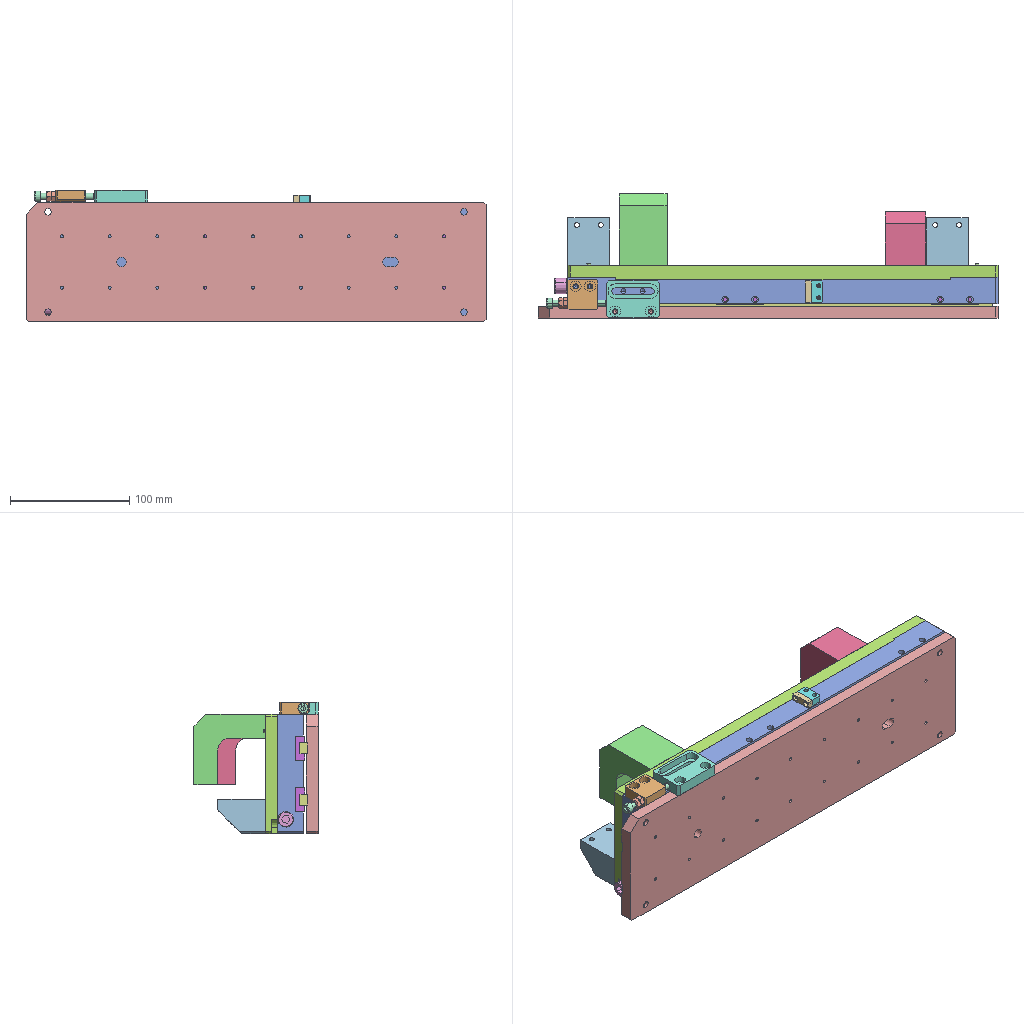Assembly | SolidWorks | 19 different items | 64 placed | box 385 x 104 x 110 mm
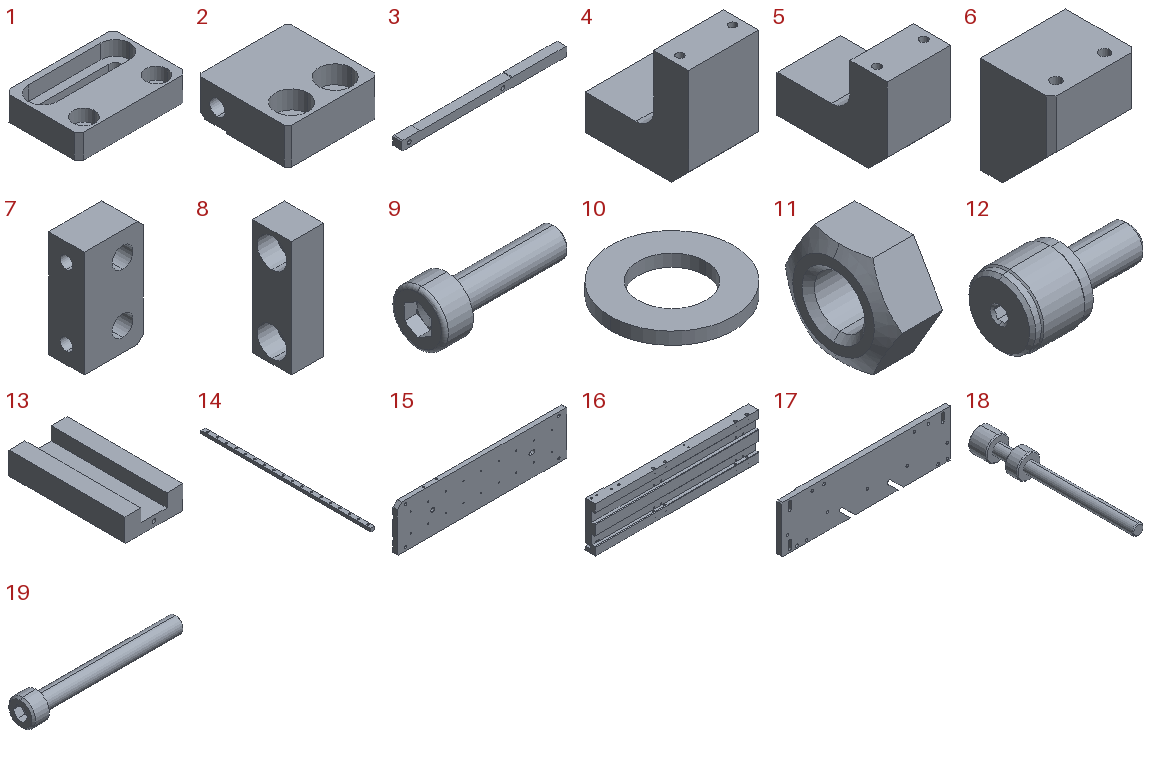Parts list (item | quantity | size | volume | features):
1 | x1 | 45 x 31 x 10 mm | 9481 mm3 | features ICE 4, Chamfer 1, Extrusion 1
2 | x1 | 25 x 25 x 10 mm | 4941 mm3 | features ICE 4, Chamfer 2, 3DProfileFeature 1, Extrusion 1, HoleWzd 1
3 | x1 | 180 x 9.8 x 10 mm | 15341 mm3 | features ICE 4, 3DProfileFeature 2, Chamfer 2, HoleWzd 2, Cut 1, Extrusion 1
4 | x1 | 40 x 59 x 60 mm | 77348 mm3 | features 3DProfileFeature 2, HoleWzd 2, Chamfer 1, Extrusion 1, Fillet 1, ICE 1
5 | x1 | 34 x 59 x 45 mm | 55439 mm3 | features 3DProfileFeature 2, HoleWzd 2, Chamfer 1, Extrusion 1, Fillet 1, ICE 1
6 | x2 | 35 x 29 x 40 mm | 32746 mm3 | features 3DProfileFeature 2, Chamfer 2, HoleWzd 2, Extrusion 1
7 | x1 | 10 x 6 x 18 mm | 923.956 mm3 | features 3DProfileFeature 1, Chamfer 1, Extrusion 1, HoleWzd 1, ICE 1
8 | x1 | 5 x 6 x 18 mm | 419.049 mm3 | features Cut 1, Extrusion 1, ICE 1
9 | x24 | 7.6 x 3 x 3 mm | 21.652 mm3 | features Fillet 2, RevCut 2, Boss 1, Chamfer 1, Cut 1, Extrusion 1, LPattern 1
10 | x16 | 10 x 10 x 1 mm | 54.782 mm3 | features Extrusion 1
11 | x2 | 4 x 9.238 x 8 mm | 160.7 mm3 | features ICE 1, RevCut 1, Revolution 1
12 | x2 | 15 x 8 x 8 mm | 435.538 mm3 | features BaseBody 1
13 | x4 | 20 x 39.9 x 8 mm | 4656 mm3 | features ICE 3, 3DProfileFeature 1, Chamfer 1, Extrusion 1, HoleWzd 1
14 | x2 | 9 x 360 x 6.5 mm | 18391 mm3 | features ICE 2, LPattern 2, Chamfer 1, Extrusion 1
15 | x1 | 385 x 10 x 100 mm | 371645 mm3 | features ICE 5, Chamfer 2, HoleWzd 2, 3DProfileFeature 1, Extrusion 1, LPattern 1
16 | x1 | 360 x 22 x 100 mm | 594910 mm3 | features ICE 9, HoleWzd 7, 3DProfileFeature 5, Chamfer 2, Fillet 2, Extrusion 1, LPattern 1, MirrorPattern 1
17 | x1 | 360 x 11.8 x 100 mm | 390446 mm3 | features ICE 12, Cut 3, Chamfer 1, Extrusion 1, LPattern 1
18 | x1 | 13 x 87 x 13 mm | 4026 mm3 | features ICE 5, Chamfer 1, Extrusion 1
19 | x1 | 50 x 8.5 x 8.5 mm | 1125 mm3 | features ICE 1, RevCut 1, Revolution 1
Mates (type | each side: item.copy, entity, surface, feature):
Coincident | 16.1 face plane Boss-Extrude1 | 17.1 face plane Boss-Extrude1 | 3 times
Coincident | 14.1 face plane Boss-Extrude1 | 13.1 face plane Cut-Extrude1 | 2 times
Coincident | 14.1 face plane Boss-Extrude1 | 13.2 face plane Cut-Extrude1
Coincident | 14.2 face plane Boss-Extrude1 | 13.3 face plane Cut-Extrude1 | 2 times
Coincident | 14.2 face plane Boss-Extrude1 | 13.4 face plane Cut-Extrude1 | 2 times
Coincident | 13.2 face plane Boss-Extrude1 | 13.4 face plane Boss-Extrude1 | 2 times
Coincident | 16.1 face plane Boss-Extrude1 | 2.1 face plane Boss-Extrude1 | 2 times
Coincident | 16.1 face plane Cut-Extrude2 | 2.1 face plane Boss-Extrude1
Concentric | 19.1 face cylinder Revolve1 | 11.1 face cylinder Cut-Revolve1
Concentric | 19.1 face cylinder Revolve1 | 11.2 face cylinder Cut-Revolve1
Concentric | 2.1 face cylinder M5 Tapped Hole1 | 19.1 face cylinder Revolve1
DistanceDim | 19.1 face plane Revolve1 | 2.1 face plane Boss-Extrude1
Coincident | 11.1 face plane Revolve1 | 11.2 face plane Revolve1
Coincident | 2.1 face plane Boss-Extrude1 | 11.1 face plane Revolve1
Coincident | 16.1 face plane Cut-Extrude5 | 18.1 face plane Boss-Extrude3
Coincident | 16.1 face plane Cut-Extrude4 | 3.1 face plane Boss-Extrude1 | 2 times
Concentric | 3.1 face cylinder M6 Tapped Hole1 | 18.1 face cylinder Boss-Extrude1
Coincident | 13.1 face plane Boss-Extrude1 | 13.3 face plane Boss-Extrude1
DistanceDim | 13.3 face plane Boss-Extrude1 | 16.1 face plane Boss-Extrude1
DistanceDim | 13.4 face plane Boss-Extrude1 | 13.3 face plane Boss-Extrude1
Concentric | 14.1 face cylinder LPattern2 | 9.1 face cylinder BaseBody
Coincident | 14.1 face plane LPattern2 | 9.1 face plane BaseHead
Concentric | 14.2 face cylinder LPattern1 | 9.2 face cylinder BaseBody
Coincident | 14.2 face plane LPattern2 | 9.2 face plane BaseHead
Coincident | 16.1 face plane Cut-Extrude8 | 10.1 face plane Base-Extrude
Concentric | 16.1 face cylinder Cut-Extrude8 | 10.1 face cylinder Base-Extrude
Coincident | 16.1 face plane Cut-Extrude8 | 10.2 face plane Base-Extrude
Concentric | 16.1 face cylinder Cut-Extrude8 | 10.2 face cylinder Base-Extrude
Coincident | 16.1 face plane Cut-Extrude8 | 10.3 face plane Base-Extrude
Concentric | 16.1 face cylinder Cut-Extrude8 | 10.3 face cylinder Base-Extrude
Coincident | 16.1 face plane Cut-Extrude8 | 10.4 face plane Base-Extrude
Concentric | 16.1 face cylinder LPattern1 | 10.4 face cylinder Base-Extrude
Coincident | 16.1 face plane Cut-Extrude8 | 10.5 face plane Base-Extrude
Concentric | 16.1 face cylinder LPattern1 | 10.5 face cylinder Base-Extrude
Coincident | 16.1 face plane Cut-Extrude8 | 10.6 face plane Base-Extrude
Concentric | 16.1 face cylinder Cut-Extrude8 | 10.6 face cylinder Base-Extrude
Coincident | 16.1 face plane Cut-Extrude8 | 10.7 face plane Base-Extrude
Concentric | 16.1 face cylinder Cut-Extrude8 | 10.7 face cylinder Base-Extrude
Coincident | 16.1 face plane Cut-Extrude8 | 10.8 face plane Base-Extrude | 2 times
Concentric | 16.1 face cylinder Cut-Extrude8 | 10.8 face cylinder Base-Extrude
Coincident | 16.1 face plane Cut-Extrude8 | 10.9 face plane Base-Extrude
Concentric | 16.1 face cylinder Cut-Extrude8 | 10.9 face cylinder Base-Extrude
Coincident | 16.1 face plane Cut-Extrude8 | 10.10 face plane Base-Extrude
Concentric | 16.1 face cylinder Cut-Extrude8 | 10.10 face cylinder Base-Extrude
Concentric | 16.1 face cylinder Cut-Extrude8 | 10.11 face cylinder Base-Extrude
Coincident | 16.1 face plane Cut-Extrude8 | 10.11 face plane Base-Extrude
Coincident | 16.1 face plane Cut-Extrude8 | 10.12 face plane Base-Extrude
Concentric | 16.1 face cylinder Cut-Extrude8 | 10.12 face cylinder Base-Extrude
Concentric | 16.1 face cylinder Cut-Extrude8 | 10.13 face cylinder Base-Extrude
Coincident | 16.1 face plane Cut-Extrude8 | 10.13 face plane Base-Extrude
Concentric | 16.1 face cylinder Cut-Extrude8 | 10.14 face cylinder Base-Extrude
Coincident | 16.1 face plane Cut-Extrude8 | 10.14 face plane Base-Extrude
Concentric | 16.1 face cylinder Cut-Extrude8 | 10.15 face cylinder Base-Extrude
Coincident | 16.1 face plane Cut-Extrude8 | 10.15 face plane Base-Extrude
Concentric | 16.1 face cylinder Cut-Extrude8 | 10.16 face cylinder Base-Extrude
Coincident | 16.1 face plane Cut-Extrude8 | 10.16 face plane Base-Extrude
Concentric | 10.15 face cylinder Base-Extrude | 9.3 face cylinder BaseBody
Coincident | 10.15 face plane Base-Extrude | 9.3 face plane BaseHead
Concentric | 16.1 face cylinder Cut-Extrude8 | 9.4 face cylinder BaseBody
Coincident | 10.16 face plane Base-Extrude | 9.4 face plane BaseHead
Concentric | 16.1 face cylinder Cut-Extrude8 | 9.5 face cylinder BaseBody
Coincident | 10.13 face plane Base-Extrude | 9.5 face plane BaseHead
Concentric | 16.1 face cylinder Cut-Extrude8 | 9.6 face cylinder BaseBody
Coincident | 10.14 face plane Base-Extrude | 9.6 face plane BaseHead
Concentric | 16.1 face cylinder Cut-Extrude8 | 9.7 face cylinder BaseBody
Coincident | 10.1 face plane Base-Extrude | 9.7 face plane BaseHead
Concentric | 16.1 face cylinder Cut-Extrude8 | 9.8 face cylinder BaseBody
Coincident | 10.11 face plane Base-Extrude | 9.8 face plane BaseHead
Concentric | 16.1 face cylinder Cut-Extrude8 | 9.9 face cylinder BaseBody
Coincident | 10.12 face plane Base-Extrude | 9.9 face plane BaseHead
Concentric | 16.1 face cylinder Cut-Extrude8 | 9.10 face cylinder BaseBody
Coincident | 10.2 face plane Base-Extrude | 9.10 face plane BaseHead
Concentric | 16.1 face cylinder LPattern1 | 9.11 face cylinder BaseBody
Coincident | 10.4 face plane Base-Extrude | 9.11 face plane BaseHead
Concentric | 10.3 face cylinder Base-Extrude | 9.12 face cylinder BaseBody
Coincident | 10.3 face plane Base-Extrude | 9.12 face plane BaseHead
Concentric | 16.1 face cylinder LPattern1 | 9.13 face cylinder BaseBody
Coincident | 10.5 face plane Base-Extrude | 9.13 face plane BaseHead
Concentric | 16.1 face cylinder Cut-Extrude8 | 9.14 face cylinder BaseBody
Coincident | 10.6 face plane Base-Extrude | 9.14 face plane BaseHead
Concentric | 16.1 face cylinder Cut-Extrude8 | 9.15 face cylinder BaseBody
Coincident | 10.8 face plane Base-Extrude | 9.15 face plane BaseHead
Concentric | 16.1 face cylinder Cut-Extrude8 | 9.16 face cylinder BaseBody
Coincident | 10.7 face plane Base-Extrude | 9.16 face plane BaseHead
Concentric | 10.10 face cylinder Base-Extrude | 9.17 face cylinder BaseBody
Coincident | 10.10 face plane Base-Extrude | 9.17 face plane BaseHead
Concentric | 16.1 face cylinder Cut-Extrude8 | 9.18 face cylinder BaseBody
Coincident | 10.9 face plane Base-Extrude | 9.18 face plane BaseHead
Coincident | 17.1 face plane Boss-Extrude1 | 4.1 face plane Boss-Extrude1 | 2 times
Concentric | 17.1 face cylinder Cut-Extrude4 | 5.1 face cylinder M5 Tapped Hole2 | 2 times
Coincident | 17.1 face plane Boss-Extrude1 | 5.1 face plane Boss-Extrude1
Concentric | 16.1 face cylinder M5 Tapped Hole1 | 9.19 face cylinder BaseBody
Concentric | 16.1 face cylinder M5 Tapped Hole2 | 9.20 face cylinder BaseBody
Concentric | 16.1 face cylinder M5 Tapped Hole3 | 9.21 face cylinder BaseBody
Coincident | 17.1 face plane Boss-Extrude1 | 9.21 face plane BaseHead
Coincident | 17.1 face plane Boss-Extrude1 | 9.20 face plane BaseHead
Coincident | 17.1 face plane Boss-Extrude1 | 9.19 face plane BaseHead
Concentric | 16.1 face cylinder M3 Tapped Hole1 | 9.22 face cylinder BaseBody
Coincident | 16.1 face plane Boss-Extrude1 | 9.22 face plane BaseHead
Concentric | 16.1 face cylinder M3 Tapped Hole1 | 9.23 face cylinder BaseBody
Coincident | 16.1 face plane Boss-Extrude1 | 9.23 face plane BaseHead
Coincident | 17.1 face plane Boss-Extrude1 | 6.1 face plane Boss-Extrude1 | 2 times
Coincident | 6.2 face plane Boss-Extrude1 | 6.1 face plane Boss-Extrude1
Concentric | 17.1 face cylinder Cut-Extrude6 | 6.2 face cylinder M5 Tapped Hole1 | 2 times
Coincident | 17.1 face plane Boss-Extrude1 | 6.2 face plane Boss-Extrude1
Coincident | 3.1 face plane Cut-Extrude4 | 12.1 face plane Input1
Concentric | 3.1 face cylinder Cut-Extrude5 | 12.1 face cylinder Input1
Coincident | 3.1 face plane Cut-Extrude4 | 12.2 face plane Input1
Concentric | 3.1 face cylinder Cut-Extrude5 | 12.2 face cylinder Input1
Tangent | 17.1 face plane Cut-Extrude2 | 12.2 face cylinder Input1
Coincident | 16.1 face plane Cut-Extrude1 | 13.3 face plane Boss-Extrude1
Concentric | 17.1 face cylinder Cut-Extrude4 | 4.1 face cylinder M5 Tapped Hole2
Coincident | 16.1 face plane Boss-Extrude1 | 7.1 face plane Boss-Extrude1
Concentric | 16.1 face cylinder M3 Tapped Hole1 | 7.1 face cylinder Cut-Extrude1 | 2 times
Coincident | 7.1 face plane Boss-Extrude1 | 8.1 face plane Boss-Extrude1 | 3 times
Concentric | 8.1 face cylinder Cut-Extrude1 | 9.24 face cylinder BaseBody
Coincident | 8.1 face plane Cut-Extrude2 | 9.24 face plane BaseHead
Coincident | 15.1 face plane Cut-Extrude1 | 14.1 face plane Boss-Extrude1
Concentric | 15.1 face cylinder LPattern1 | 14.1 face cylinder LPattern2 | 2 times
Coincident | 15.1 face plane Cut-Extrude1 | 14.2 face plane Boss-Extrude1
Concentric | 15.1 face cylinder LPattern1 | 14.2 face cylinder LPattern2
Coincident | 15.1 face plane Boss-Extrude1 | 1.1 face plane Boss-Extrude1
Concentric | 15.1 face cylinder M4 Tapped Hole1 | 1.1 face cylinder Cut-Extrude2 | 2 times
Coincident | 15.1 face plane Boss-Extrude1 | 16.1 face plane Boss-Extrude1 | 2 times